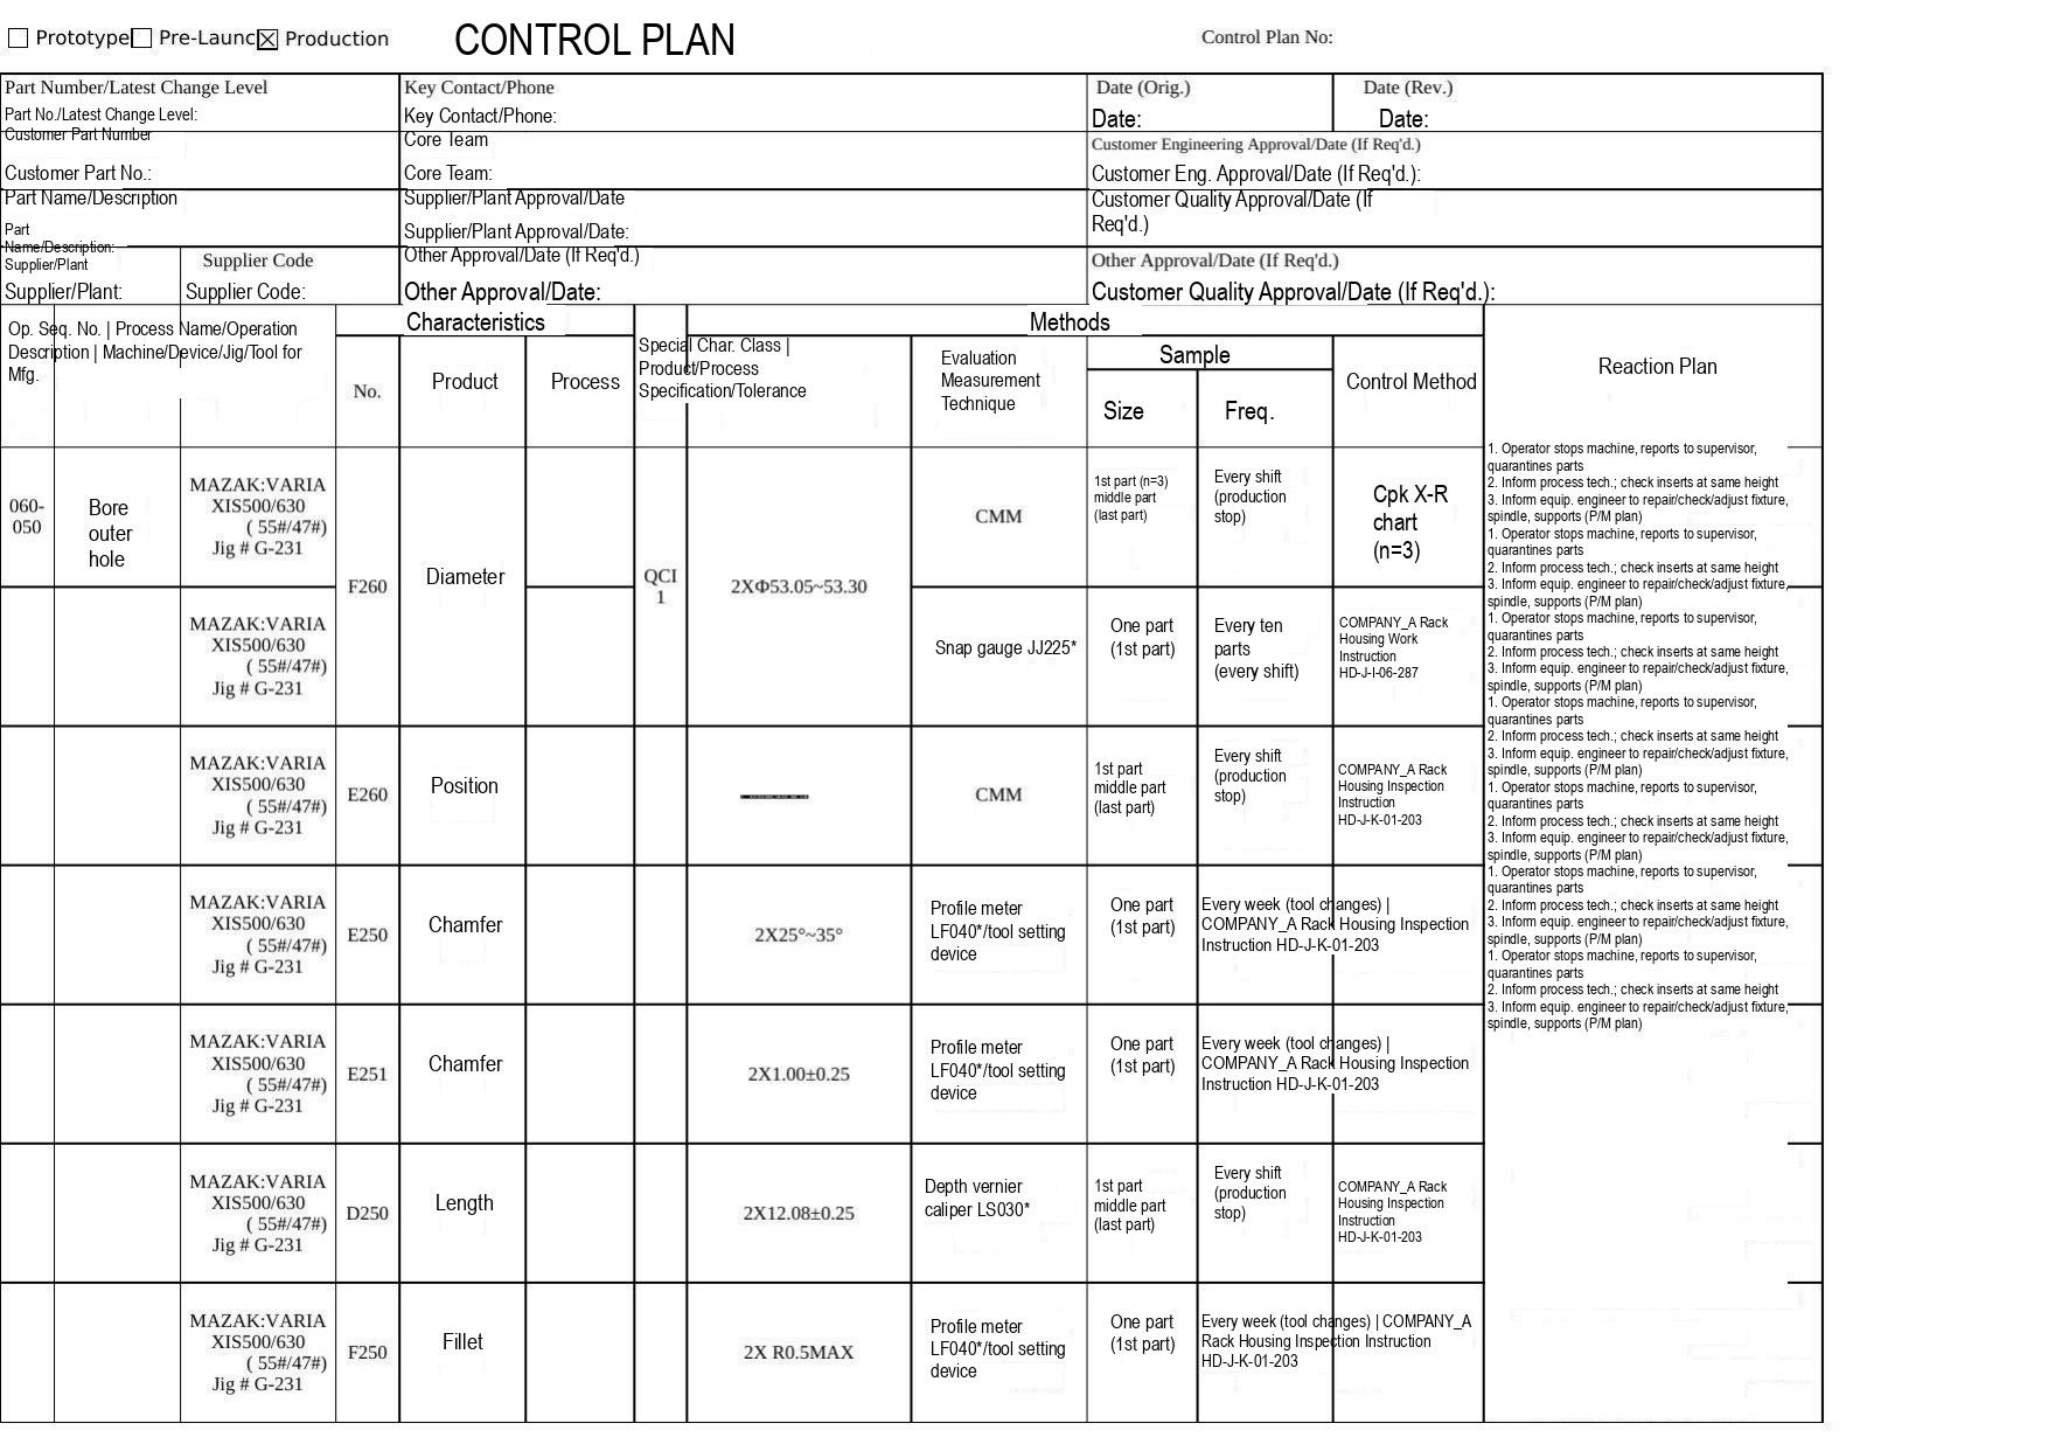☐ Prototype☐ Pre-Launc☒ Production

# CONTROL PLAN

Control Plan No:

| Part Number/Latest Change Level | Key Contact/Phone | Date (Orig.) | Date (Rev.) |
|---|---|---|---|
| Part No./Latest Change Level: | Key Contact/Phone: | Date: | Date: |
| Customer Part Number<br>Customer Part No.: | Core Team<br>Core Team: | Customer Engineering Approval/Date (If Req'd.)<br>Customer Eng. Approval/Date (If Req'd.): | |
| Part Name/Description<br>Part Name/Description: | Supplier/Plant Approval/Date<br>Supplier/Plant Approval/Date: | Customer Quality Approval/Date (If Req'd.) | |
| Supplier/Plant<br>Supplier/Plant: — Supplier Code<br>Supplier Code: | Other Approval/Date (If Req'd.)<br>Other Approval/Date: | Other Approval/Date (If Req'd.)<br>Customer Quality Approval/Date (If Req'd.): | |

| Op. Seq. No. | Process Name/Operation Description | Machine/Device/Jig/Tool for Mfg. | Characteristics No. | Characteristics Product | Characteristics Process | Special Char. Class | Product/Process Specification/Tolerance | Methods Evaluation Measurement Technique | Sample Size | Sample Freq. | Control Method | Reaction Plan |
|---|---|---|---|---|---|---|---|---|---|---|---|---|
| 060-050 | Bore outer hole | MAZAK:VARIA XIS500/630 ( 55#/47#) Jig # G-231 | F260 | Diameter | | QCI 1 | 2XΦ53.05~53.30 | CMM | 1st part (n=3) middle part (last part) | Every shift (production stop) | Cpk X-R chart (n=3) | 1. Operator stops machine, reports to supervisor, quarantines parts 2. Inform process tech.; check inserts at same height 3. Inform equip. engineer to repair/check/adjust fixture, spindle, supports (P/M plan) |
| | | MAZAK:VARIA XIS500/630 ( 55#/47#) Jig # G-231 | | | | | | Snap gauge JJ225* | One part (1st part) | Every ten parts (every shift) | COMPANY_A Rack Housing Work Instruction HD-J-I-06-287 | 1. Operator stops machine, reports to supervisor, quarantines parts 2. Inform process tech.; check inserts at same height 3. Inform equip. engineer to repair/check/adjust fixture, spindle, supports (P/M plan) |
| | | MAZAK:VARIA XIS500/630 ( 55#/47#) Jig # G-231 | E260 | Position | | | | CMM | 1st part middle part (last part) | Every shift (production stop) | COMPANY_A Rack Housing Inspection Instruction HD-J-K-01-203 | 1. Operator stops machine, reports to supervisor, quarantines parts 2. Inform process tech.; check inserts at same height 3. Inform equip. engineer to repair/check/adjust fixture, spindle, supports (P/M plan) |
| | | MAZAK:VARIA XIS500/630 ( 55#/47#) Jig # G-231 | E250 | Chamfer | | | 2X25°~35° | Profile meter LF040*/tool setting device | One part (1st part) | Every week (tool changes) | COMPANY_A Rack Housing Inspection Instruction HD-J-K-01-203 | 1. Operator stops machine, reports to supervisor, quarantines parts 2. Inform process tech.; check inserts at same height 3. Inform equip. engineer to repair/check/adjust fixture, spindle, supports (P/M plan) |
| | | MAZAK:VARIA XIS500/630 ( 55#/47#) Jig # G-231 | E251 | Chamfer | | | 2X1.00±0.25 | Profile meter LF040*/tool setting device | One part (1st part) | Every week (tool changes) | COMPANY_A Rack Housing Inspection Instruction HD-J-K-01-203 | 1. Operator stops machine, reports to supervisor, quarantines parts 2. Inform process tech.; check inserts at same height 3. Inform equip. engineer to repair/check/adjust fixture, spindle, supports (P/M plan) |
| | | MAZAK:VARIA XIS500/630 ( 55#/47#) Jig # G-231 | D250 | Length | | | 2X12.08±0.25 | Depth vernier caliper LS030* | 1st part middle part (last part) | Every shift (production stop) | COMPANY_A Rack Housing Inspection Instruction HD-J-K-01-203 | 1. Operator stops machine, reports to supervisor, quarantines parts 2. Inform process tech.; check inserts at same height 3. Inform equip. engineer to repair/check/adjust fixture, spindle, supports (P/M plan) |
| | | MAZAK:VARIA XIS500/630 ( 55#/47#) Jig # G-231 | F250 | Fillet | | | 2X R0.5MAX | Profile meter LF040*/tool setting device | One part (1st part) | Every week (tool changes) | COMPANY_A Rack Housing Inspection Instruction HD-J-K-01-203 | |
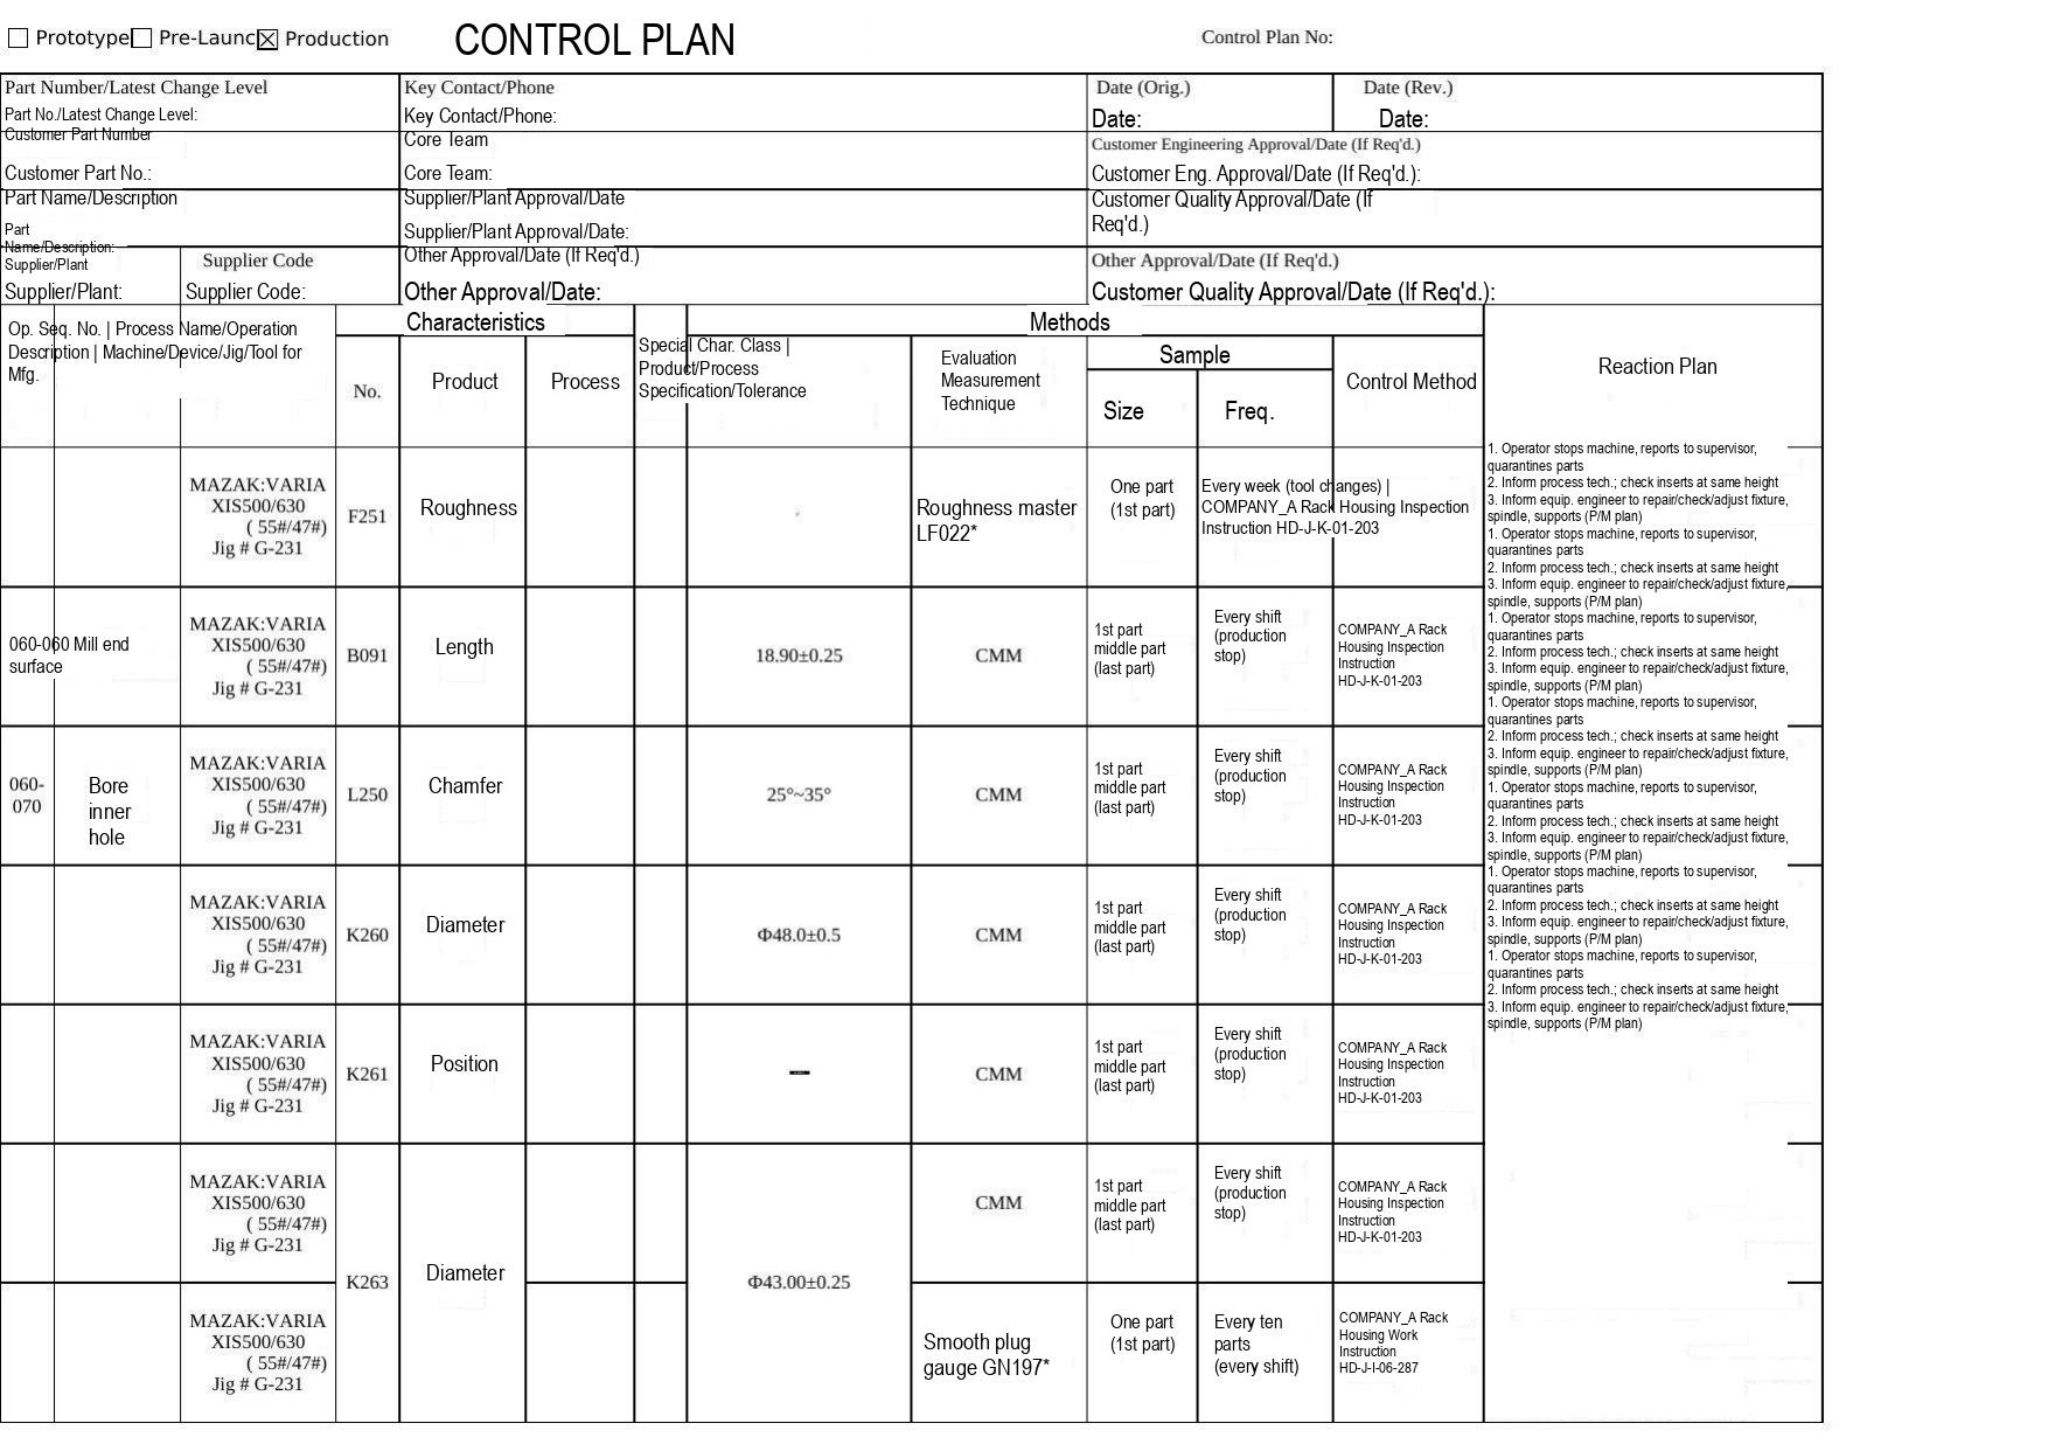☐ Prototype ☐ Pre-Launc ☒ Production

# CONTROL PLAN

Control Plan No:

| Part Number/Latest Change Level<br>Part No./Latest Change Level: | Key Contact/Phone<br>Key Contact/Phone: | Date (Orig.)<br>Date: | Date (Rev.)<br>Date: |
|---|---|---|---|
| Customer Part Number<br>Customer Part No.: | Core Team<br>Core Team: | Customer Engineering Approval/Date (If Req'd.)<br>Customer Eng. Approval/Date (If Req'd.): | |
| Part Name/Description<br>Part Name/Description: | Supplier/Plant Approval/Date<br>Supplier/Plant Approval/Date: | Customer Quality Approval/Date (If Req'd.) | |
| Supplier/Plant<br>Supplier/Plant: / Supplier Code<br>Supplier Code: | Other Approval/Date (If Req'd.)<br>Other Approval/Date: | Other Approval/Date (If Req'd.)<br>Customer Quality Approval/Date (If Req'd.): | |

| Op. Seq. No. | Process Name/Operation Description | Machine/Device/Jig/Tool for Mfg. | No. (Characteristics) | Product (Characteristics) | Process (Characteristics) | Special Char. Class | Product/Process Specification/Tolerance (Methods) | Evaluation Measurement Technique (Methods) | Sample Size (Methods) | Sample Freq. (Methods) | Control Method (Methods) | Reaction Plan |
|---|---|---|---|---|---|---|---|---|---|---|---|---|
| | | MAZAK:VARIA XIS500/630 ( 55#/47#) Jig # G-231 | F251 | Roughness | | | | Roughness master LF022* | One part (1st part) | Every week (tool changes) | COMPANY_A Rack Housing Inspection Instruction HD-J-K-01-203 | 1. Operator stops machine, reports to supervisor, quarantines parts 2. Inform process tech.; check inserts at same height 3. Inform equip. engineer to repair/check/adjust fixture, spindle, supports (P/M plan) |
| 060-060 | Mill end surface | MAZAK:VARIA XIS500/630 ( 55#/47#) Jig # G-231 | B091 | Length | | | 18.90±0.25 | CMM | 1st part middle part (last part) | Every shift (production stop) | COMPANY_A Rack Housing Inspection Instruction HD-J-K-01-203 | 1. Operator stops machine, reports to supervisor, quarantines parts 2. Inform process tech.; check inserts at same height 3. Inform equip. engineer to repair/check/adjust fixture, spindle, supports (P/M plan) |
| 060-070 | Bore inner hole | MAZAK:VARIA XIS500/630 ( 55#/47#) Jig # G-231 | L250 | Chamfer | | | 25°~35° | CMM | 1st part middle part (last part) | Every shift (production stop) | COMPANY_A Rack Housing Inspection Instruction HD-J-K-01-203 | 1. Operator stops machine, reports to supervisor, quarantines parts 2. Inform process tech.; check inserts at same height 3. Inform equip. engineer to repair/check/adjust fixture, spindle, supports (P/M plan) |
| | | MAZAK:VARIA XIS500/630 ( 55#/47#) Jig # G-231 | K260 | Diameter | | | Φ48.0±0.5 | CMM | 1st part middle part (last part) | Every shift (production stop) | COMPANY_A Rack Housing Inspection Instruction HD-J-K-01-203 | 1. Operator stops machine, reports to supervisor, quarantines parts 2. Inform process tech.; check inserts at same height 3. Inform equip. engineer to repair/check/adjust fixture, spindle, supports (P/M plan) |
| | | MAZAK:VARIA XIS500/630 ( 55#/47#) Jig # G-231 | K261 | Position | | | — | CMM | 1st part middle part (last part) | Every shift (production stop) | COMPANY_A Rack Housing Inspection Instruction HD-J-K-01-203 | 1. Operator stops machine, reports to supervisor, quarantines parts 2. Inform process tech.; check inserts at same height 3. Inform equip. engineer to repair/check/adjust fixture, spindle, supports (P/M plan) |
| | | MAZAK:VARIA XIS500/630 ( 55#/47#) Jig # G-231 | K263 | Diameter | | | Φ43.00±0.25 | CMM | 1st part middle part (last part) | Every shift (production stop) | COMPANY_A Rack Housing Inspection Instruction HD-J-K-01-203 | 1. Operator stops machine, reports to supervisor, quarantines parts 2. Inform process tech.; check inserts at same height 3. Inform equip. engineer to repair/check/adjust fixture, spindle, supports (P/M plan) |
| | | MAZAK:VARIA XIS500/630 ( 55#/47#) Jig # G-231 | K263 | Diameter | | | Φ43.00±0.25 | Smooth plug gauge GN197* | One part (1st part) | Every ten parts (every shift) | COMPANY_A Rack Housing Work Instruction HD-J-I-06-287 | 1. Operator stops machine, reports to supervisor, quarantines parts 2. Inform process tech.; check inserts at same height 3. Inform equip. engineer to repair/check/adjust fixture, spindle, supports (P/M plan) |
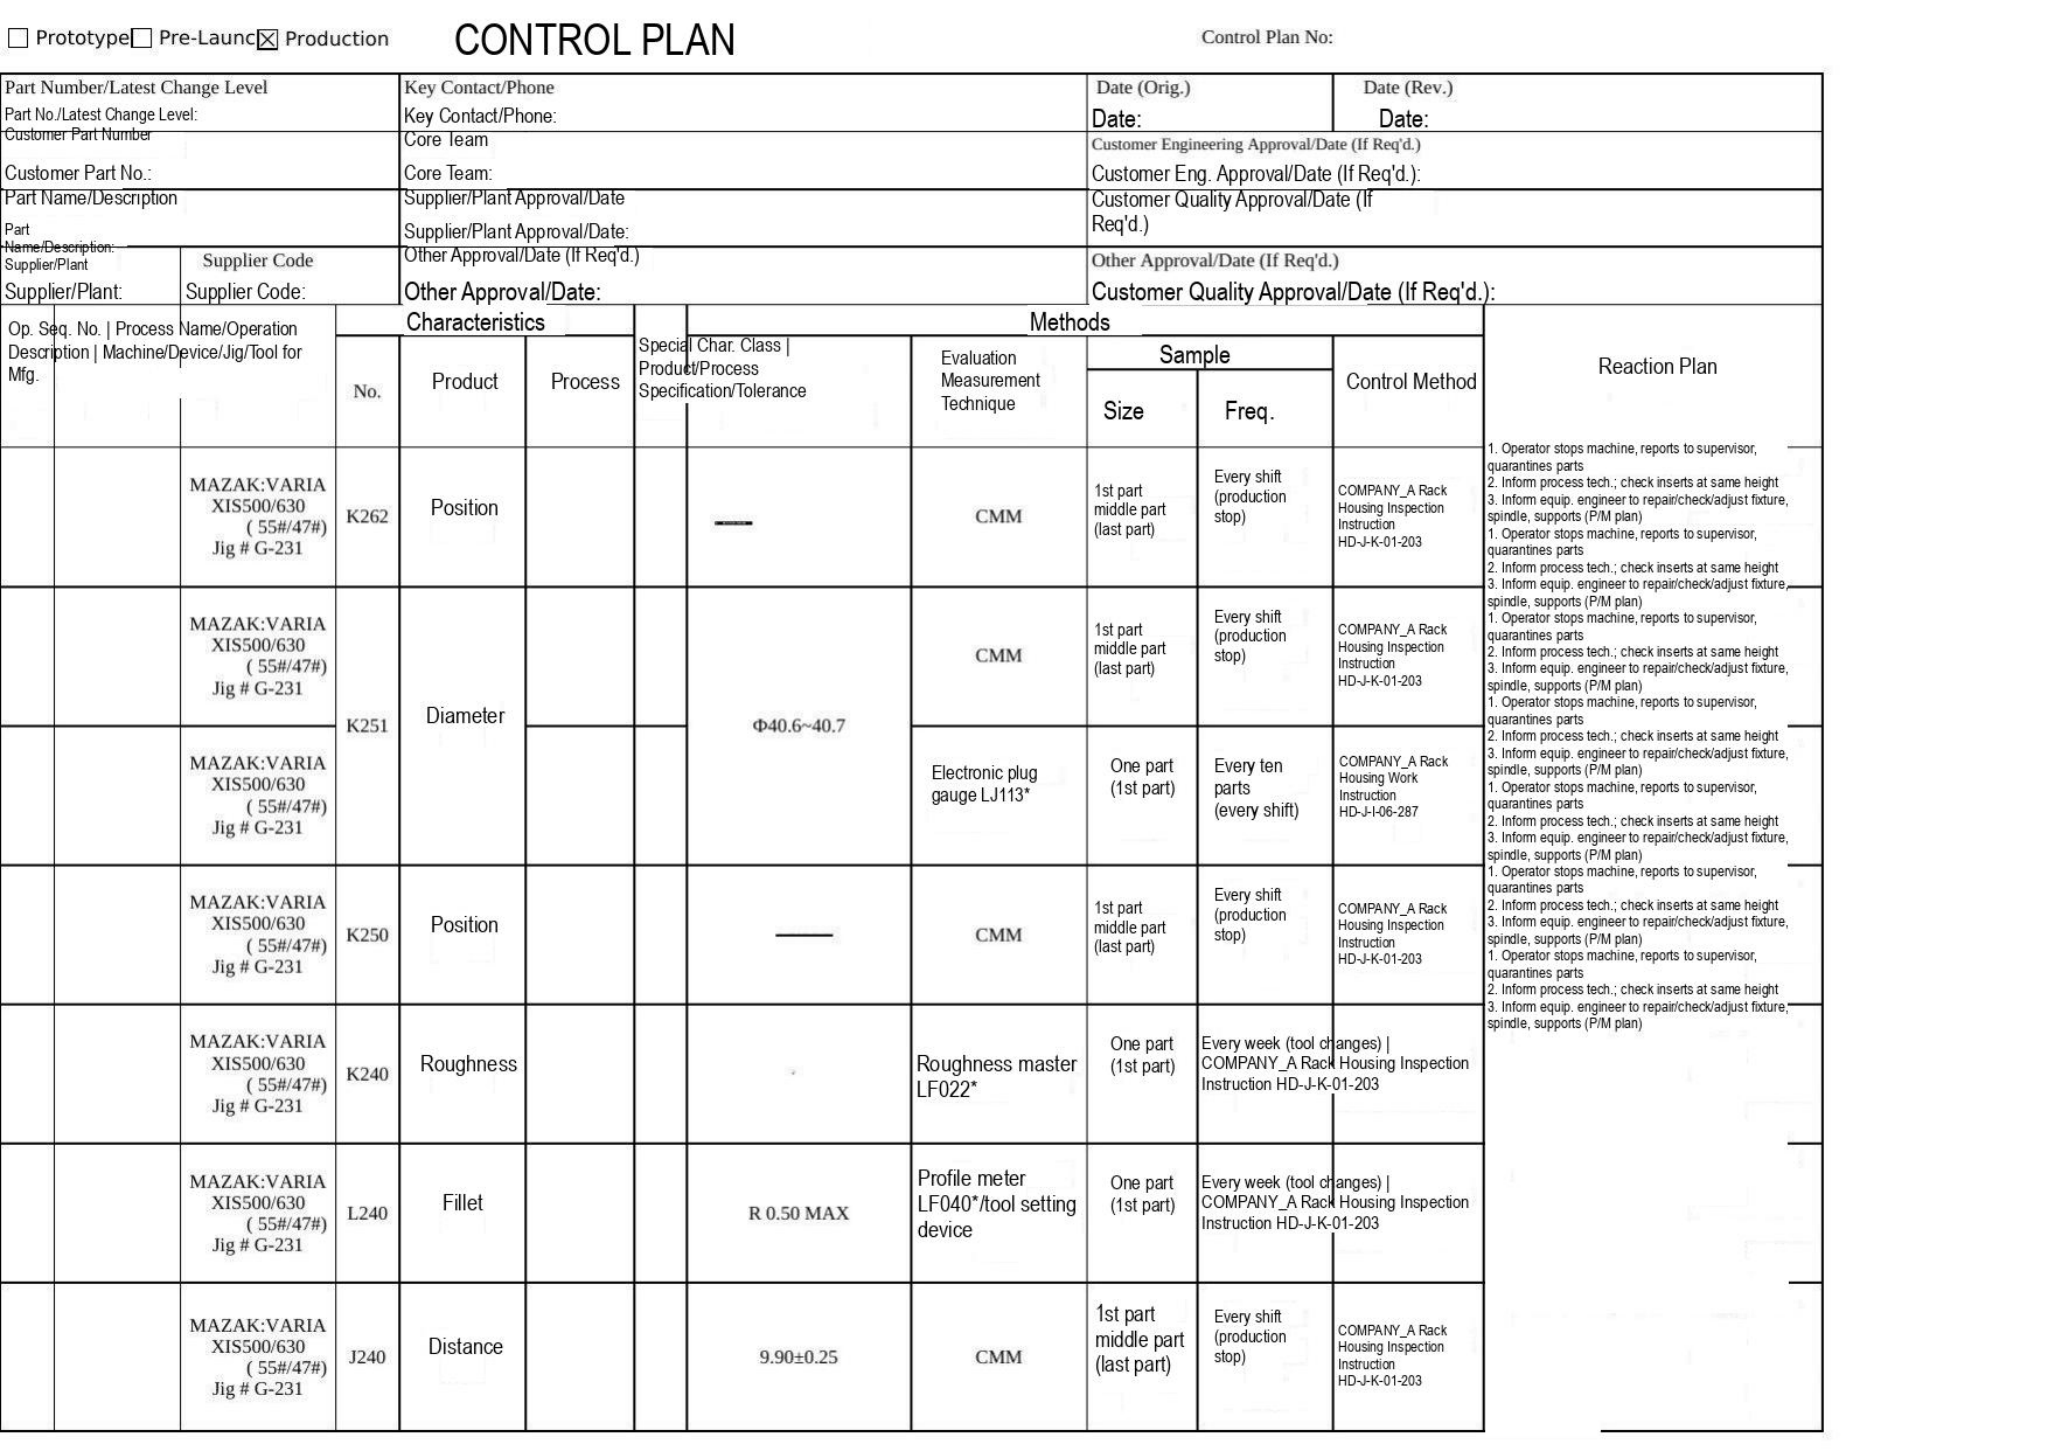☐ Prototype☐ Pre-Launc☒ Production

# CONTROL PLAN

Control Plan No:

| Part Number/Latest Change Level | | Key Contact/Phone | Date (Orig.) | Date (Rev.) |
|---|---|---|---|---|
| Part No./Latest Change Level: | | Key Contact/Phone: | Date: | Date: |
| Customer Part Number | | Core Team | Customer Engineering Approval/Date (If Req'd.) | |
| Customer Part No.: | | Core Team: | Customer Eng. Approval/Date (If Req'd.): | |
| Part Name/Description | | Supplier/Plant Approval/Date | Customer Quality Approval/Date (If Req'd.) | |
| Part Name/Description: | | Supplier/Plant Approval/Date: | | |
| Supplier/Plant | Supplier Code | Other Approval/Date (If Req'd.) | Other Approval/Date (If Req'd.) | |
| Supplier/Plant: | Supplier Code: | Other Approval/Date: | Customer Quality Approval/Date (If Req'd.): | |

| Op. Seq. No. | Process Name/Operation Description | Machine/Device/Jig/Tool for Mfg. | Characteristics No. | Characteristics Product | Characteristics Process | Special Char. Class | Product/Process Specification/Tolerance | Methods Evaluation Measurement Technique | Methods Sample Size | Methods Sample Freq. | Methods Control Method | Reaction Plan |
|---|---|---|---|---|---|---|---|---|---|---|---|---|
| | | MAZAK:VARIA XIS500/630 ( 55#/47#) Jig # G-231 | K262 | Position | | | —— | CMM | 1st part middle part (last part) | Every shift (production stop) | COMPANY_A Rack Housing Inspection Instruction HD-J-K-01-203 | 1. Operator stops machine, reports to supervisor, quarantines parts 2. Inform process tech.; check inserts at same height 3. Inform equip. engineer to repair/check/adjust fixture, spindle, supports (P/M plan) |
| | | MAZAK:VARIA XIS500/630 ( 55#/47#) Jig # G-231 | K251 | Diameter | | | Φ40.6~40.7 | CMM | 1st part middle part (last part) | Every shift (production stop) | COMPANY_A Rack Housing Inspection Instruction HD-J-K-01-203 | 1. Operator stops machine, reports to supervisor, quarantines parts 2. Inform process tech.; check inserts at same height 3. Inform equip. engineer to repair/check/adjust fixture, spindle, supports (P/M plan) |
| | | MAZAK:VARIA XIS500/630 ( 55#/47#) Jig # G-231 | | | | | | Electronic plug gauge LJ113* | One part (1st part) | Every ten parts (every shift) | COMPANY_A Rack Housing Work Instruction HD-J-I-06-287 | 1. Operator stops machine, reports to supervisor, quarantines parts 2. Inform process tech.; check inserts at same height 3. Inform equip. engineer to repair/check/adjust fixture, spindle, supports (P/M plan) |
| | | MAZAK:VARIA XIS500/630 ( 55#/47#) Jig # G-231 | K250 | Position | | | —— | CMM | 1st part middle part (last part) | Every shift (production stop) | COMPANY_A Rack Housing Inspection Instruction HD-J-K-01-203 | 1. Operator stops machine, reports to supervisor, quarantines parts 2. Inform process tech.; check inserts at same height 3. Inform equip. engineer to repair/check/adjust fixture, spindle, supports (P/M plan) |
| | | MAZAK:VARIA XIS500/630 ( 55#/47#) Jig # G-231 | K240 | Roughness | | | | Roughness master LF022* | One part (1st part) | Every week (tool changes) | COMPANY_A Rack Housing Inspection Instruction HD-J-K-01-203 | 1. Operator stops machine, reports to supervisor, quarantines parts 2. Inform process tech.; check inserts at same height 3. Inform equip. engineer to repair/check/adjust fixture, spindle, supports (P/M plan) |
| | | MAZAK:VARIA XIS500/630 ( 55#/47#) Jig # G-231 | L240 | Fillet | | | R 0.50 MAX | Profile meter LF040*/tool setting device | One part (1st part) | Every week (tool changes) | COMPANY_A Rack Housing Inspection Instruction HD-J-K-01-203 | 1. Operator stops machine, reports to supervisor, quarantines parts 2. Inform process tech.; check inserts at same height 3. Inform equip. engineer to repair/check/adjust fixture, spindle, supports (P/M plan) |
| | | MAZAK:VARIA XIS500/630 ( 55#/47#) Jig # G-231 | J240 | Distance | | | 9.90±0.25 | CMM | 1st part middle part (last part) | Every shift (production stop) | COMPANY_A Rack Housing Inspection Instruction HD-J-K-01-203 | 1. Operator stops machine, reports to supervisor, quarantines parts 2. Inform process tech.; check inserts at same height 3. Inform equip. engineer to repair/check/adjust fixture, spindle, supports (P/M plan) |
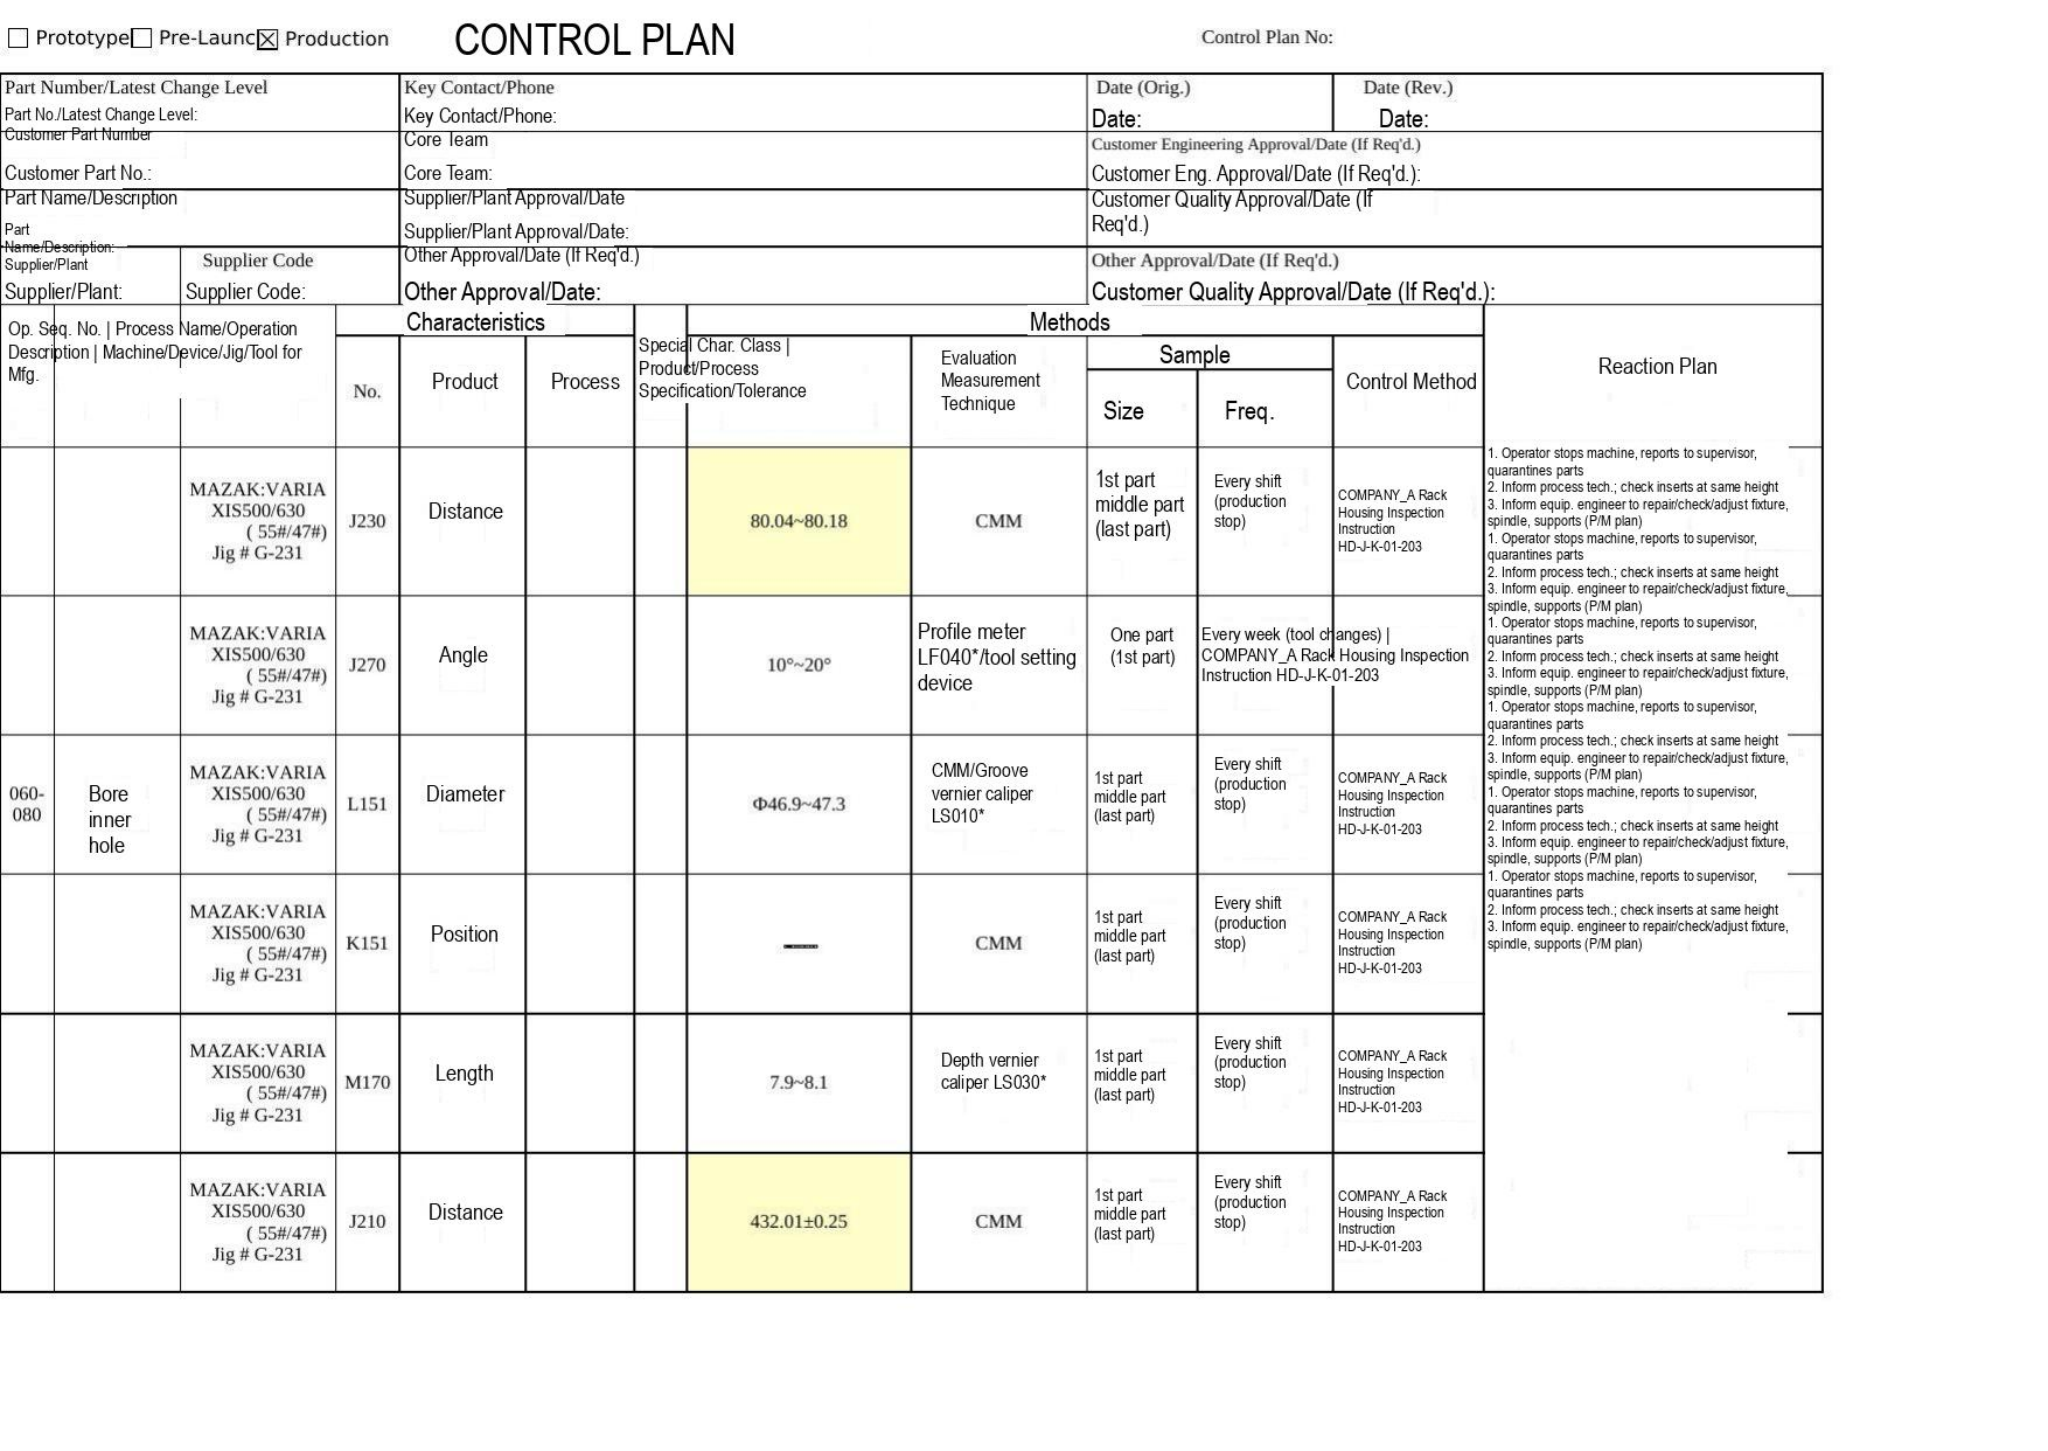☐ Prototype☐ Pre-Launc☒ Production

CONTROL PLAN

Control Plan No:

| Part Number/Latest Change Level<br>Part No./Latest Change Level: | | Key Contact/Phone<br>Key Contact/Phone: | Date (Orig.)<br>Date: | Date (Rev.)<br>Date: |
|---|---|---|---|---|
| Customer Part Number<br>Customer Part No.: | | Core Team<br>Core Team: | Customer Engineering Approval/Date (If Req'd.)<br>Customer Eng. Approval/Date (If Req'd.): | |
| Part Name/Description<br>Part Name/Description: | | Supplier/Plant Approval/Date<br>Supplier/Plant Approval/Date: | Customer Quality Approval/Date (If Req'd.) | |
| Supplier/Plant<br>Supplier/Plant: | Supplier Code<br>Supplier Code: | Other Approval/Date (If Req'd.)<br>Other Approval/Date: | Other Approval/Date (If Req'd.)<br>Customer Quality Approval/Date (If Req'd.): | |

| Op. Seq. No. \| Process Name/Operation Description \| Machine/Device/Jig/Tool for Mfg. | | | Characteristics<br>No. | Characteristics<br>Product | Characteristics<br>Process | Special Char. Class \| Product/Process Specification/Tolerance | | Methods<br>Evaluation Measurement Technique | Sample<br>Size | Sample<br>Freq. | Control Method | Reaction Plan |
|---|---|---|---|---|---|---|---|---|---|---|---|---|
| | | MAZAK:VARIA XIS500/630 ( 55#/47#) Jig # G-231 | J230 | Distance | | | 80.04~80.18 | CMM | 1st part middle part (last part) | Every shift (production stop) | COMPANY_A Rack Housing Inspection Instruction HD-J-K-01-203 | 1. Operator stops machine, reports to supervisor, quarantines parts 2. Inform process tech.; check inserts at same height 3. Inform equip. engineer to repair/check/adjust fixture, spindle, supports (P/M plan) |
| | | MAZAK:VARIA XIS500/630 ( 55#/47#) Jig # G-231 | J270 | Angle | | | 10°~20° | Profile meter LF040*/tool setting device | One part (1st part) | Every week (tool changes) | COMPANY_A Rack Housing Inspection Instruction HD-J-K-01-203 | 1. Operator stops machine, reports to supervisor, quarantines parts 2. Inform process tech.; check inserts at same height 3. Inform equip. engineer to repair/check/adjust fixture, spindle, supports (P/M plan) |
| 060-080 | Bore inner hole | MAZAK:VARIA XIS500/630 ( 55#/47#) Jig # G-231 | L151 | Diameter | | | Φ46.9~47.3 | CMM/Groove vernier caliper LS010* | 1st part middle part (last part) | Every shift (production stop) | COMPANY_A Rack Housing Inspection Instruction HD-J-K-01-203 | 1. Operator stops machine, reports to supervisor, quarantines parts 2. Inform process tech.; check inserts at same height 3. Inform equip. engineer to repair/check/adjust fixture, spindle, supports (P/M plan) |
| | | MAZAK:VARIA XIS500/630 ( 55#/47#) Jig # G-231 | K151 | Position | | | — | CMM | 1st part middle part (last part) | Every shift (production stop) | COMPANY_A Rack Housing Inspection Instruction HD-J-K-01-203 | 1. Operator stops machine, reports to supervisor, quarantines parts 2. Inform process tech.; check inserts at same height 3. Inform equip. engineer to repair/check/adjust fixture, spindle, supports (P/M plan) |
| | | MAZAK:VARIA XIS500/630 ( 55#/47#) Jig # G-231 | M170 | Length | | | 7.9~8.1 | Depth vernier caliper LS030* | 1st part middle part (last part) | Every shift (production stop) | COMPANY_A Rack Housing Inspection Instruction HD-J-K-01-203 | 1. Operator stops machine, reports to supervisor, quarantines parts 2. Inform process tech.; check inserts at same height 3. Inform equip. engineer to repair/check/adjust fixture, spindle, supports (P/M plan) |
| | | MAZAK:VARIA XIS500/630 ( 55#/47#) Jig # G-231 | J210 | Distance | | | 432.01±0.25 | CMM | 1st part middle part (last part) | Every shift (production stop) | COMPANY_A Rack Housing Inspection Instruction HD-J-K-01-203 | 1. Operator stops machine, reports to supervisor, quarantines parts 2. Inform process tech.; check inserts at same height 3. Inform equip. engineer to repair/check/adjust fixture, spindle, supports (P/M plan) |
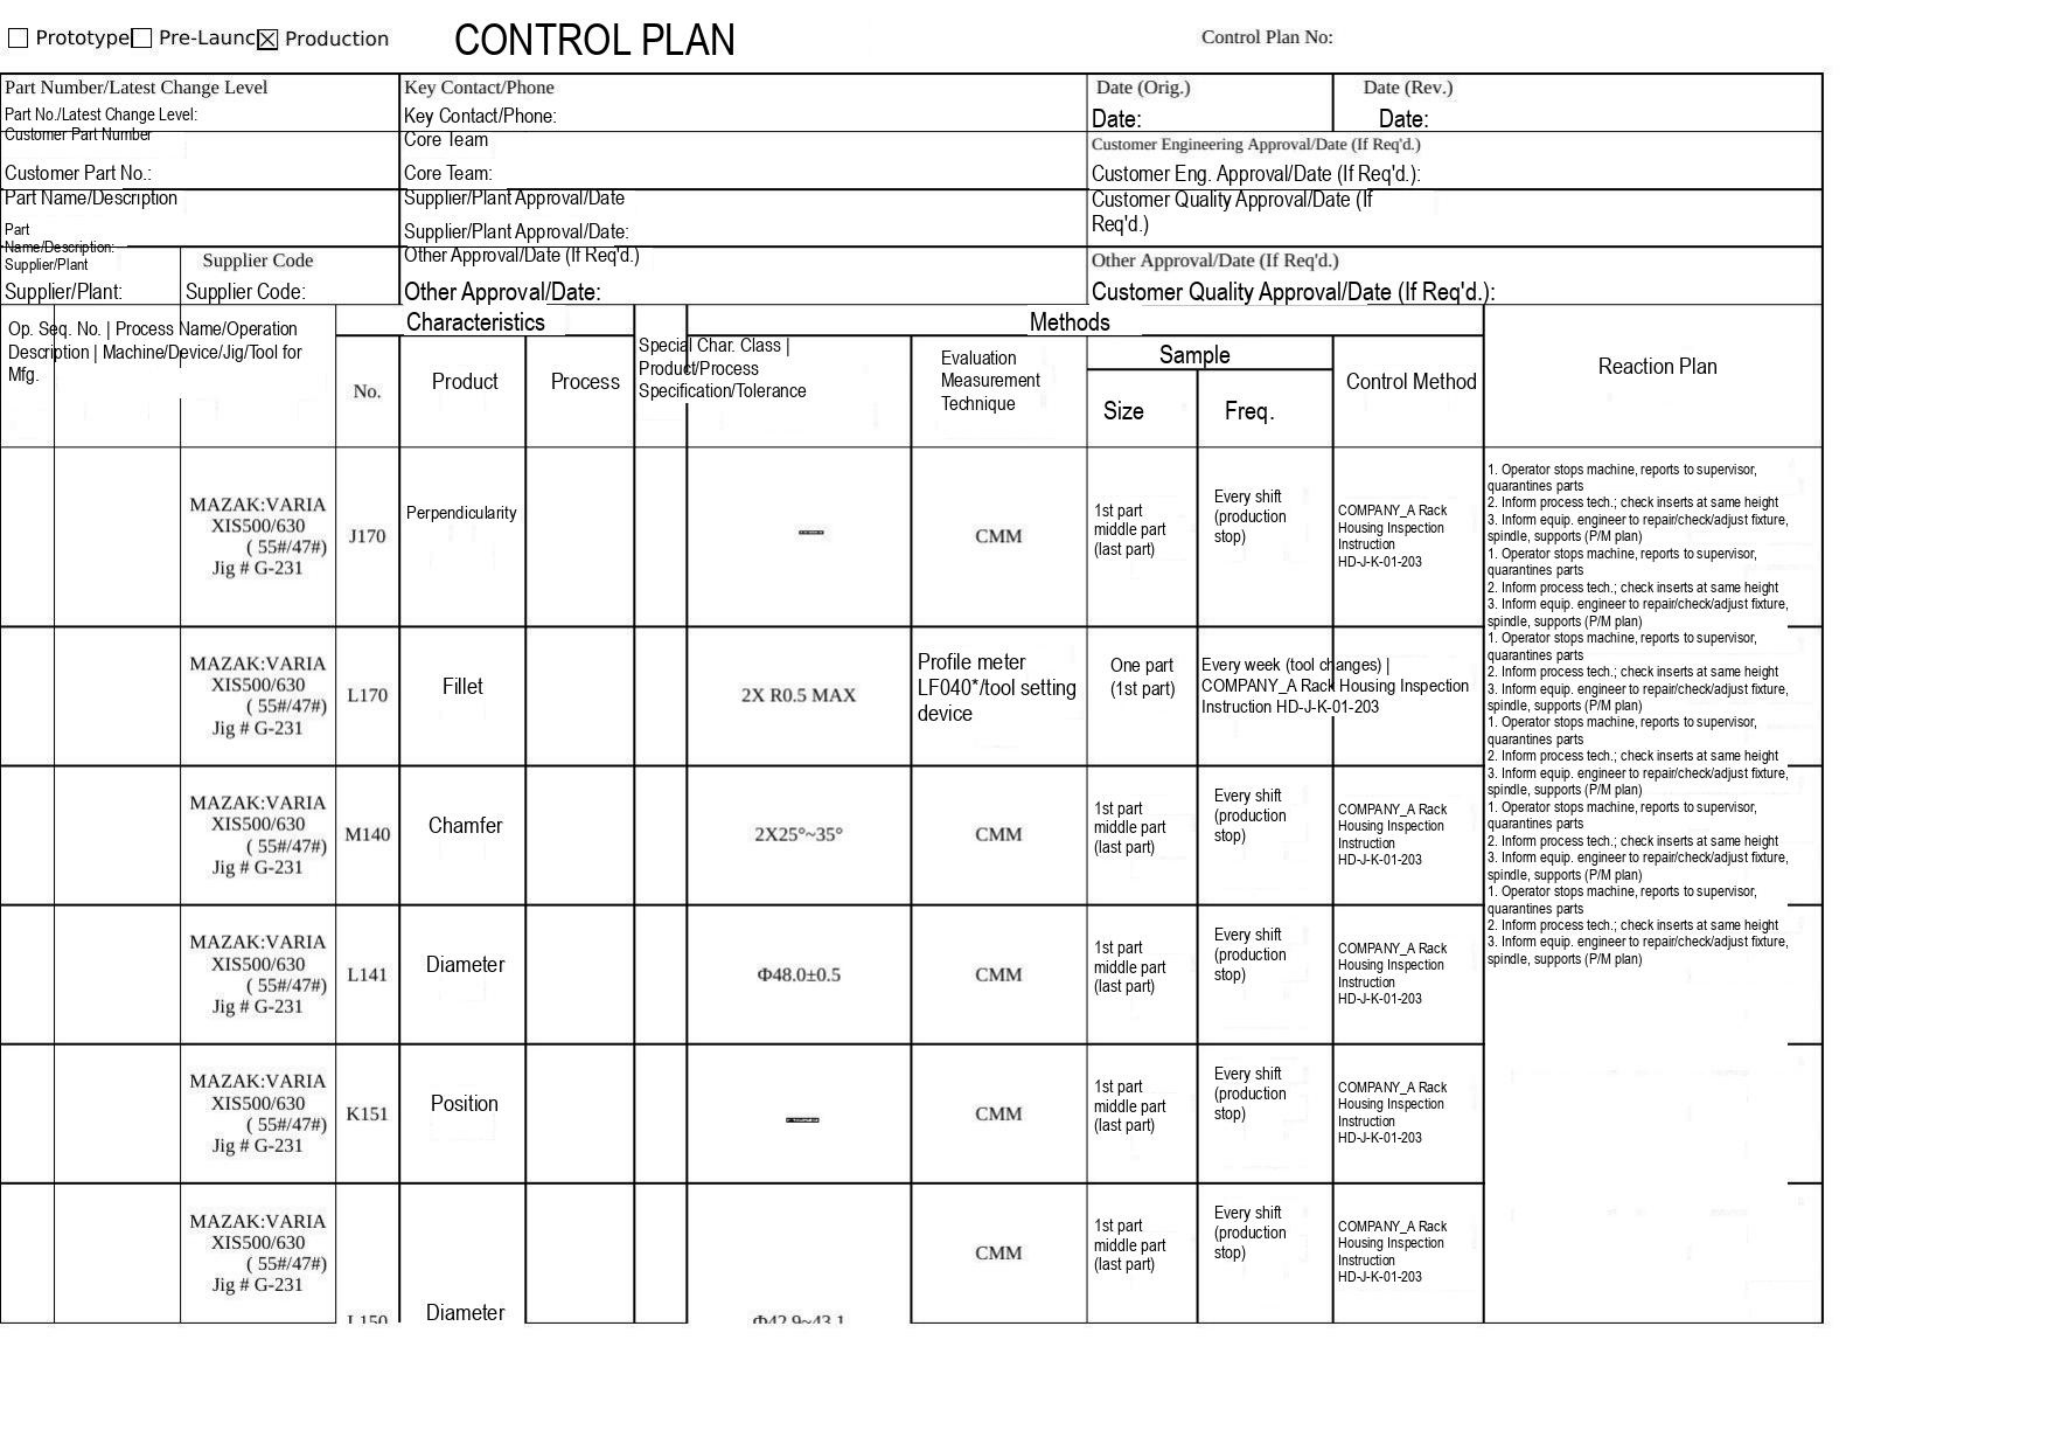☐ Prototype ☐ Pre-Launch ☒ Production

# CONTROL PLAN

Control Plan No:

| Part Number/Latest Change Level<br>Part No./Latest Change Level: | Key Contact/Phone<br>Key Contact/Phone: | Date (Orig.)<br>Date: | Date (Rev.)<br>Date: |
|---|---|---|---|
| Customer Part Number<br>Customer Part No.: | Core Team<br>Core Team: | Customer Engineering Approval/Date (If Req'd.)<br>Customer Eng. Approval/Date (If Req'd.): | |
| Part Name/Description<br>Part Name/Description: | Supplier/Plant Approval/Date<br>Supplier/Plant Approval/Date: | Customer Quality Approval/Date (If Req'd.) | |
| Supplier/Plant<br>Supplier/Plant: / Supplier Code<br>Supplier Code: | Other Approval/Date (If Req'd.)<br>Other Approval/Date: | Other Approval/Date (If Req'd.)<br>Customer Quality Approval/Date (If Req'd.): | |

| Op. Seq. No. \| Process Name/Operation Description \| Machine/Device/Jig/Tool for Mfg. | | | Characteristics: No. | Characteristics: Product | Characteristics: Process | Methods: Special Char. Class \| Product/Process Specification/Tolerance | | Methods: Evaluation Measurement Technique | Methods: Sample Size | Methods: Sample Freq. | Methods: Control Method | Reaction Plan |
|---|---|---|---|---|---|---|---|---|---|---|---|---|
| | | MAZAK:VARIAXIS500/630 ( 55#/47#) Jig # G-231 | J170 | Perpendicularity | | | | CMM | 1st part middle part (last part) | Every shift (production stop) | COMPANY_A Rack Housing Inspection Instruction HD-J-K-01-203 | 1. Operator stops machine, reports to supervisor, quarantines parts 2. Inform process tech.; check inserts at same height 3. Inform equip. engineer to repair/check/adjust fixture, spindle, supports (P/M plan) 1. Operator stops machine, reports to supervisor, quarantines parts 2. Inform process tech.; check inserts at same height 3. Inform equip. engineer to repair/check/adjust fixture, spindle, supports (P/M plan) |
| | | MAZAK:VARIAXIS500/630 ( 55#/47#) Jig # G-231 | L170 | Fillet | | | 2X R0.5 MAX | Profile meter LF040*/tool setting device | One part (1st part) | Every week (tool changes) \| COMPANY_A Rack Housing Inspection Instruction HD-J-K-01-203 | | 1. Operator stops machine, reports to supervisor, quarantines parts 2. Inform process tech.; check inserts at same height 3. Inform equip. engineer to repair/check/adjust fixture, spindle, supports (P/M plan) 1. Operator stops machine, reports to supervisor, quarantines parts 2. Inform process tech.; check inserts at same height 3. Inform equip. engineer to repair/check/adjust fixture, spindle, supports (P/M plan) |
| | | MAZAK:VARIAXIS500/630 ( 55#/47#) Jig # G-231 | M140 | Chamfer | | | 2X25°~35° | CMM | 1st part middle part (last part) | Every shift (production stop) | COMPANY_A Rack Housing Inspection Instruction HD-J-K-01-203 | 1. Operator stops machine, reports to supervisor, quarantines parts 2. Inform process tech.; check inserts at same height 3. Inform equip. engineer to repair/check/adjust fixture, spindle, supports (P/M plan) |
| | | MAZAK:VARIAXIS500/630 ( 55#/47#) Jig # G-231 | L141 | Diameter | | | Φ48.0±0.5 | CMM | 1st part middle part (last part) | Every shift (production stop) | COMPANY_A Rack Housing Inspection Instruction HD-J-K-01-203 | 1. Operator stops machine, reports to supervisor, quarantines parts 2. Inform process tech.; check inserts at same height 3. Inform equip. engineer to repair/check/adjust fixture, spindle, supports (P/M plan) |
| | | MAZAK:VARIAXIS500/630 ( 55#/47#) Jig # G-231 | K151 | Position | | | | CMM | 1st part middle part (last part) | Every shift (production stop) | COMPANY_A Rack Housing Inspection Instruction HD-J-K-01-203 | |
| | | MAZAK:VARIAXIS500/630 ( 55#/47#) Jig # G-231 | L150 | Diameter | | | Φ42.9~43.1 | CMM | 1st part middle part (last part) | Every shift (production stop) | COMPANY_A Rack Housing Inspection Instruction HD-J-K-01-203 | |